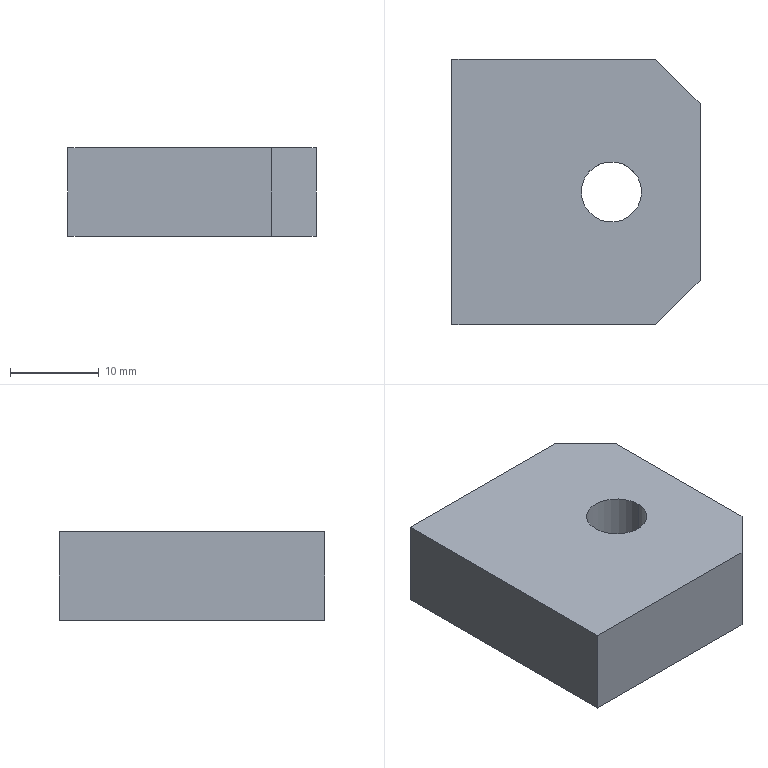Part | SolidWorks | features BaseBody 1 | 1 solid | 10 faces | box 28 x 30 x 10 mm | volume 7787 mm3 | plane 8 | cylinder 2 | commonest cylinder face diameters 6.8 x2
STEP:
#1=CARTESIAN_POINT('',(7.4,0.,10.));
#2=VERTEX_POINT('',#1);
#3=CARTESIAN_POINT('',(7.4,0.,0.));
#4=VERTEX_POINT('',#3);
#5=CARTESIAN_POINT('',(7.4,0.,0.));
#6=DIRECTION('',(0.,0.,-1.));
#7=VECTOR('',#6,1000.);
#8=LINE('',#5,#7);
#9=EDGE_CURVE('',#2,#4,#8,.T.);
#10=ORIENTED_EDGE('',*,*,#9,.F.);
#11=CARTESIAN_POINT('',(0.6,0.,10.));
#12=VERTEX_POINT('',#11);
#13=CARTESIAN_POINT('',(4.,0.,10.));
#14=DIRECTION('',(0.,0.,1.));
#15=DIRECTION('',(1.,0.,0.));
#16=AXIS2_PLACEMENT_3D('',#13,#14,#15);
#17=CIRCLE('',#16,3.4);
#18=EDGE_CURVE('',#2,#12,#17,.T.);
#19=ORIENTED_EDGE('',*,*,#18,.T.);
#20=CARTESIAN_POINT('',(0.6,0.,0.));
#21=VERTEX_POINT('',#20);
#22=CARTESIAN_POINT('',(0.6,0.,0.));
#23=DIRECTION('',(0.,0.,-1.));
#24=VECTOR('',#23,1000.);
#25=LINE('',#22,#24);
#26=EDGE_CURVE('',#12,#21,#25,.T.);
#27=ORIENTED_EDGE('',*,*,#26,.T.);
#28=CARTESIAN_POINT('',(4.,0.,0.));
#29=DIRECTION('',(0.,0.,-1.));
#30=DIRECTION('',(-1.,0.,0.));
#31=AXIS2_PLACEMENT_3D('',#28,#29,#30);
#32=CIRCLE('',#31,3.4);
#33=EDGE_CURVE('',#21,#4,#32,.T.);
#34=ORIENTED_EDGE('',*,*,#33,.T.);
#35=EDGE_LOOP('',(#10,#19,#27,#34));
#36=FACE_OUTER_BOUND('',#35,.T.);
#37=CARTESIAN_POINT('',(4.,0.,0.));
#38=DIRECTION('',(0.,0.,-1.));
#39=DIRECTION('',(-1.,0.,0.));
#40=AXIS2_PLACEMENT_3D('',#37,#38,#39);
#41=CYLINDRICAL_SURFACE('',#40,3.4);
#42=ADVANCED_FACE('',(#36),#41,.F.);
#43=CARTESIAN_POINT('',(14.,10.,10.));
#44=VERTEX_POINT('',#43);
#45=CARTESIAN_POINT('',(9.,15.,10.));
#46=VERTEX_POINT('',#45);
#47=CARTESIAN_POINT('',(12.,12.,10.));
#48=DIRECTION('',(-0.7071,0.7071,0.));
#49=VECTOR('',#48,1000.);
#50=LINE('',#47,#49);
#51=EDGE_CURVE('',#44,#46,#50,.T.);
#52=ORIENTED_EDGE('',*,*,#51,.F.);
#53=CARTESIAN_POINT('',(14.,10.,0.));
#54=VERTEX_POINT('',#53);
#55=CARTESIAN_POINT('',(14.,10.,10.));
#56=DIRECTION('',(0.,0.,1.));
#57=VECTOR('',#56,1000.);
#58=LINE('',#55,#57);
#59=EDGE_CURVE('',#54,#44,#58,.T.);
#60=ORIENTED_EDGE('',*,*,#59,.F.);
#61=CARTESIAN_POINT('',(9.,15.,0.));
#62=VERTEX_POINT('',#61);
#63=CARTESIAN_POINT('',(9.,15.,0.));
#64=DIRECTION('',(0.7071,-0.7071,0.));
#65=VECTOR('',#64,1000.);
#66=LINE('',#63,#65);
#67=EDGE_CURVE('',#62,#54,#66,.T.);
#68=ORIENTED_EDGE('',*,*,#67,.F.);
#69=CARTESIAN_POINT('',(9.,15.,10.));
#70=DIRECTION('',(0.,0.,-1.));
#71=VECTOR('',#70,1000.);
#72=LINE('',#69,#71);
#73=EDGE_CURVE('',#46,#62,#72,.T.);
#74=ORIENTED_EDGE('',*,*,#73,.F.);
#75=EDGE_LOOP('',(#52,#60,#68,#74));
#76=FACE_OUTER_BOUND('',#75,.T.);
#77=CARTESIAN_POINT('',(9.,15.,10.));
#78=DIRECTION('',(-0.7071,-0.7071,0.));
#79=DIRECTION('',(-0.7071,0.7071,0.));
#80=AXIS2_PLACEMENT_3D('',#77,#78,#79);
#81=PLANE('',#80);
#82=ADVANCED_FACE('',(#76),#81,.F.);
#83=CARTESIAN_POINT('',(9.,-15.,10.));
#84=VERTEX_POINT('',#83);
#85=CARTESIAN_POINT('',(14.,-10.,10.));
#86=VERTEX_POINT('',#85);
#87=CARTESIAN_POINT('',(12.,-12.,10.));
#88=DIRECTION('',(0.7071,0.7071,0.));
#89=VECTOR('',#88,1000.);
#90=LINE('',#87,#89);
#91=EDGE_CURVE('',#84,#86,#90,.T.);
#92=ORIENTED_EDGE('',*,*,#91,.F.);
#93=CARTESIAN_POINT('',(9.,-15.,0.));
#94=VERTEX_POINT('',#93);
#95=CARTESIAN_POINT('',(9.,-15.,10.));
#96=DIRECTION('',(0.,0.,1.));
#97=VECTOR('',#96,1000.);
#98=LINE('',#95,#97);
#99=EDGE_CURVE('',#94,#84,#98,.T.);
#100=ORIENTED_EDGE('',*,*,#99,.F.);
#101=CARTESIAN_POINT('',(14.,-10.,0.));
#102=VERTEX_POINT('',#101);
#103=CARTESIAN_POINT('',(14.,-10.,0.));
#104=DIRECTION('',(-0.7071,-0.7071,0.));
#105=VECTOR('',#104,1000.);
#106=LINE('',#103,#105);
#107=EDGE_CURVE('',#102,#94,#106,.T.);
#108=ORIENTED_EDGE('',*,*,#107,.F.);
#109=CARTESIAN_POINT('',(14.,-10.,10.));
#110=DIRECTION('',(0.,0.,-1.));
#111=VECTOR('',#110,1000.);
#112=LINE('',#109,#111);
#113=EDGE_CURVE('',#86,#102,#112,.T.);
#114=ORIENTED_EDGE('',*,*,#113,.F.);
#115=EDGE_LOOP('',(#92,#100,#108,#114));
#116=FACE_OUTER_BOUND('',#115,.T.);
#117=CARTESIAN_POINT('',(14.,-10.,10.));
#118=DIRECTION('',(-0.7071,0.7071,0.));
#119=DIRECTION('',(0.,0.,1.));
#120=AXIS2_PLACEMENT_3D('',#117,#118,#119);
#121=PLANE('',#120);
#122=ADVANCED_FACE('',(#116),#121,.F.);
#123=ORIENTED_EDGE('',*,*,#33,.F.);
#124=CARTESIAN_POINT('',(4.,0.,0.));
#125=DIRECTION('',(0.,0.,-1.));
#126=DIRECTION('',(-1.,0.,0.));
#127=AXIS2_PLACEMENT_3D('',#124,#125,#126);
#128=CIRCLE('',#127,3.4);
#129=EDGE_CURVE('',#4,#21,#128,.T.);
#130=ORIENTED_EDGE('',*,*,#129,.F.);
#131=EDGE_LOOP('',(#123,#130));
#132=FACE_BOUND('',#131,.T.);
#133=CARTESIAN_POINT('',(14.,-15.,0.));
#134=DIRECTION('',(0.,1.,0.));
#135=VECTOR('',#134,1000.);
#136=LINE('',#133,#135);
#137=EDGE_CURVE('',#102,#54,#136,.T.);
#138=ORIENTED_EDGE('',*,*,#137,.F.);
#139=ORIENTED_EDGE('',*,*,#107,.T.);
#140=CARTESIAN_POINT('',(-14.,-15.,0.));
#141=VERTEX_POINT('',#140);
#142=CARTESIAN_POINT('',(14.,-15.,0.));
#143=DIRECTION('',(1.,0.,0.));
#144=VECTOR('',#143,1000.);
#145=LINE('',#142,#144);
#146=EDGE_CURVE('',#141,#94,#145,.T.);
#147=ORIENTED_EDGE('',*,*,#146,.F.);
#148=CARTESIAN_POINT('',(-14.,15.,0.));
#149=VERTEX_POINT('',#148);
#150=CARTESIAN_POINT('',(-14.,-15.,0.));
#151=DIRECTION('',(0.,-1.,0.));
#152=VECTOR('',#151,1000.);
#153=LINE('',#150,#152);
#154=EDGE_CURVE('',#149,#141,#153,.T.);
#155=ORIENTED_EDGE('',*,*,#154,.F.);
#156=CARTESIAN_POINT('',(14.,15.,0.));
#157=DIRECTION('',(-1.,0.,0.));
#158=VECTOR('',#157,1000.);
#159=LINE('',#156,#158);
#160=EDGE_CURVE('',#62,#149,#159,.T.);
#161=ORIENTED_EDGE('',*,*,#160,.F.);
#162=ORIENTED_EDGE('',*,*,#67,.T.);
#163=EDGE_LOOP('',(#138,#139,#147,#155,#161,#162));
#164=FACE_OUTER_BOUND('',#163,.T.);
#165=CARTESIAN_POINT('',(0.,0.,0.));
#166=DIRECTION('',(0.,0.,1.));
#167=DIRECTION('',(1.,0.,0.));
#168=AXIS2_PLACEMENT_3D('',#165,#166,#167);
#169=PLANE('',#168);
#170=ADVANCED_FACE('',(#132,#164),#169,.F.);
#171=CARTESIAN_POINT('',(4.,0.,10.));
#172=DIRECTION('',(0.,0.,1.));
#173=DIRECTION('',(1.,0.,0.));
#174=AXIS2_PLACEMENT_3D('',#171,#172,#173);
#175=CIRCLE('',#174,3.4);
#176=EDGE_CURVE('',#12,#2,#175,.T.);
#177=ORIENTED_EDGE('',*,*,#176,.F.);
#178=ORIENTED_EDGE('',*,*,#18,.F.);
#179=EDGE_LOOP('',(#177,#178));
#180=FACE_BOUND('',#179,.T.);
#181=CARTESIAN_POINT('',(-14.,-15.,10.));
#182=VERTEX_POINT('',#181);
#183=CARTESIAN_POINT('',(14.,-15.,10.));
#184=DIRECTION('',(1.,0.,0.));
#185=VECTOR('',#184,1000.);
#186=LINE('',#183,#185);
#187=EDGE_CURVE('',#182,#84,#186,.T.);
#188=ORIENTED_EDGE('',*,*,#187,.T.);
#189=ORIENTED_EDGE('',*,*,#91,.T.);
#190=CARTESIAN_POINT('',(14.,-15.,10.));
#191=DIRECTION('',(0.,1.,0.));
#192=VECTOR('',#191,1000.);
#193=LINE('',#190,#192);
#194=EDGE_CURVE('',#86,#44,#193,.T.);
#195=ORIENTED_EDGE('',*,*,#194,.T.);
#196=ORIENTED_EDGE('',*,*,#51,.T.);
#197=CARTESIAN_POINT('',(-14.,15.,10.));
#198=VERTEX_POINT('',#197);
#199=CARTESIAN_POINT('',(14.,15.,10.));
#200=DIRECTION('',(-1.,0.,0.));
#201=VECTOR('',#200,1000.);
#202=LINE('',#199,#201);
#203=EDGE_CURVE('',#46,#198,#202,.T.);
#204=ORIENTED_EDGE('',*,*,#203,.T.);
#205=CARTESIAN_POINT('',(-14.,-15.,10.));
#206=DIRECTION('',(0.,-1.,0.));
#207=VECTOR('',#206,1000.);
#208=LINE('',#205,#207);
#209=EDGE_CURVE('',#198,#182,#208,.T.);
#210=ORIENTED_EDGE('',*,*,#209,.T.);
#211=EDGE_LOOP('',(#188,#189,#195,#196,#204,#210));
#212=FACE_OUTER_BOUND('',#211,.T.);
#213=CARTESIAN_POINT('',(0.,0.,10.));
#214=DIRECTION('',(0.,0.,1.));
#215=DIRECTION('',(1.,0.,0.));
#216=AXIS2_PLACEMENT_3D('',#213,#214,#215);
#217=PLANE('',#216);
#218=ADVANCED_FACE('',(#180,#212),#217,.T.);
#219=ORIENTED_EDGE('',*,*,#203,.F.);
#220=ORIENTED_EDGE('',*,*,#73,.T.);
#221=ORIENTED_EDGE('',*,*,#160,.T.);
#222=CARTESIAN_POINT('',(-14.,15.,10.));
#223=DIRECTION('',(0.,0.,-1.));
#224=VECTOR('',#223,1000.);
#225=LINE('',#222,#224);
#226=EDGE_CURVE('',#198,#149,#225,.T.);
#227=ORIENTED_EDGE('',*,*,#226,.F.);
#228=EDGE_LOOP('',(#219,#220,#221,#227));
#229=FACE_OUTER_BOUND('',#228,.T.);
#230=CARTESIAN_POINT('',(14.,15.,10.));
#231=DIRECTION('',(0.,-1.,0.));
#232=DIRECTION('',(0.,0.,-1.));
#233=AXIS2_PLACEMENT_3D('',#230,#231,#232);
#234=PLANE('',#233);
#235=ADVANCED_FACE('',(#229),#234,.F.);
#236=ORIENTED_EDGE('',*,*,#194,.F.);
#237=ORIENTED_EDGE('',*,*,#113,.T.);
#238=ORIENTED_EDGE('',*,*,#137,.T.);
#239=ORIENTED_EDGE('',*,*,#59,.T.);
#240=EDGE_LOOP('',(#236,#237,#238,#239));
#241=FACE_OUTER_BOUND('',#240,.T.);
#242=CARTESIAN_POINT('',(14.,-15.,10.));
#243=DIRECTION('',(-1.,0.,0.));
#244=DIRECTION('',(0.,0.,1.));
#245=AXIS2_PLACEMENT_3D('',#242,#243,#244);
#246=PLANE('',#245);
#247=ADVANCED_FACE('',(#241),#246,.F.);
#248=ORIENTED_EDGE('',*,*,#146,.T.);
#249=ORIENTED_EDGE('',*,*,#99,.T.);
#250=ORIENTED_EDGE('',*,*,#187,.F.);
#251=CARTESIAN_POINT('',(-14.,-15.,10.));
#252=DIRECTION('',(0.,0.,-1.));
#253=VECTOR('',#252,1000.);
#254=LINE('',#251,#253);
#255=EDGE_CURVE('',#182,#141,#254,.T.);
#256=ORIENTED_EDGE('',*,*,#255,.T.);
#257=EDGE_LOOP('',(#248,#249,#250,#256));
#258=FACE_OUTER_BOUND('',#257,.T.);
#259=CARTESIAN_POINT('',(14.,-15.,10.));
#260=DIRECTION('',(0.,1.,0.));
#261=DIRECTION('',(1.,0.,0.));
#262=AXIS2_PLACEMENT_3D('',#259,#260,#261);
#263=PLANE('',#262);
#264=ADVANCED_FACE('',(#258),#263,.F.);
#265=ORIENTED_EDGE('',*,*,#154,.T.);
#266=ORIENTED_EDGE('',*,*,#255,.F.);
#267=ORIENTED_EDGE('',*,*,#209,.F.);
#268=ORIENTED_EDGE('',*,*,#226,.T.);
#269=EDGE_LOOP('',(#265,#266,#267,#268));
#270=FACE_OUTER_BOUND('',#269,.T.);
#271=CARTESIAN_POINT('',(-14.,-15.,10.));
#272=DIRECTION('',(1.,0.,0.));
#273=DIRECTION('',(0.,1.,0.));
#274=AXIS2_PLACEMENT_3D('',#271,#272,#273);
#275=PLANE('',#274);
#276=ADVANCED_FACE('',(#270),#275,.F.);
#277=ORIENTED_EDGE('',*,*,#176,.T.);
#278=ORIENTED_EDGE('',*,*,#9,.T.);
#279=ORIENTED_EDGE('',*,*,#129,.T.);
#280=ORIENTED_EDGE('',*,*,#26,.F.);
#281=EDGE_LOOP('',(#277,#278,#279,#280));
#282=FACE_OUTER_BOUND('',#281,.T.);
#283=CARTESIAN_POINT('',(4.,0.,0.));
#284=DIRECTION('',(0.,0.,-1.));
#285=DIRECTION('',(-1.,0.,0.));
#286=AXIS2_PLACEMENT_3D('',#283,#284,#285);
#287=CYLINDRICAL_SURFACE('',#286,3.4);
#288=ADVANCED_FACE('',(#282),#287,.F.);
#289=CLOSED_SHELL('',(#42,#82,#122,#170,#218,#235,#247,#264,#276,#288));
#290=MANIFOLD_SOLID_BREP('',#289);
#291=CARTESIAN_POINT('',(0.,0.,0.));
#292=DIRECTION('',(0.,0.,1.));
#293=DIRECTION('',(1.,0.,0.));
#294=AXIS2_PLACEMENT_3D('',#291,#292,#293);
#295=(LENGTH_UNIT()NAMED_UNIT(*)SI_UNIT(.MILLI.,.METRE.));
#296=UNCERTAINTY_MEASURE_WITH_UNIT(LENGTH_MEASURE(0.00001),#295,'','');
#297=(NAMED_UNIT(*)PLANE_ANGLE_UNIT()SI_UNIT($,.RADIAN.));
#298=(NAMED_UNIT(*)SI_UNIT($,.STERADIAN.)SOLID_ANGLE_UNIT());
#299=(GEOMETRIC_REPRESENTATION_CONTEXT(3)GLOBAL_UNCERTAINTY_ASSIGNED_CONTEXT((#296))GLOBAL_UNIT_ASSIGNED_CONTEXT((#295,#297,#298))REPRESENTATION_CONTEXT('',''));
#300=ADVANCED_BREP_SHAPE_REPRESENTATION('',(#290,#294),#299);